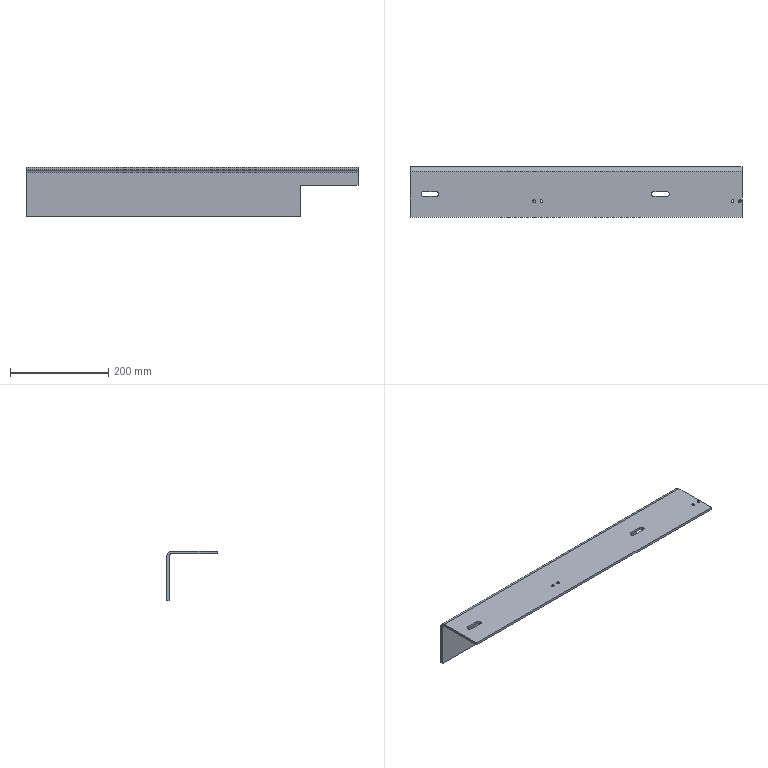Part | NX | 1 solid | 38 faces | box 677.4 x 103.1 x 101 mm | volume 622204 mm3 | cylinder 16 | plane 14 | cone 8 | commonest cylinder face diameters 5 x8 10 x7 20 x1
STEP:
#1=CARTESIAN_POINT('',(626.7,130.8,34.5));
#2=VERTEX_POINT('',#1);
#3=CARTESIAN_POINT('',(626.7,223.9,34.5));
#4=VERTEX_POINT('',#3);
#5=CARTESIAN_POINT('',(626.7,141.246,34.5));
#6=DIRECTION('',(0.,1.,0.));
#7=VECTOR('',#6,1000.);
#8=LINE('',#5,#7);
#9=EDGE_CURVE('',#2,#4,#8,.T.);
#10=ORIENTED_EDGE('',*,*,#9,.F.);
#11=CARTESIAN_POINT('',(626.7,130.8,29.5));
#12=VERTEX_POINT('',#11);
#13=CARTESIAN_POINT('',(626.7,130.8,29.5));
#14=DIRECTION('',(0.,0.,1.));
#15=VECTOR('',#14,1000.);
#16=LINE('',#13,#15);
#17=EDGE_CURVE('',#12,#2,#16,.T.);
#18=ORIENTED_EDGE('',*,*,#17,.F.);
#19=CARTESIAN_POINT('',(626.7,223.9,29.5));
#20=VERTEX_POINT('',#19);
#21=CARTESIAN_POINT('',(626.7,141.246,29.5));
#22=DIRECTION('',(0.,1.,0.));
#23=VECTOR('',#22,1000.);
#24=LINE('',#21,#23);
#25=EDGE_CURVE('',#12,#20,#24,.T.);
#26=ORIENTED_EDGE('',*,*,#25,.T.);
#27=CARTESIAN_POINT('',(626.7,228.9,24.5));
#28=VERTEX_POINT('',#27);
#29=CARTESIAN_POINT('',(626.7,223.9,24.5));
#30=DIRECTION('',(1.,0.,0.));
#31=DIRECTION('',(0.,-1.,0.));
#32=AXIS2_PLACEMENT_3D('',#29,#30,#31);
#33=CIRCLE('',#32,5.);
#34=EDGE_CURVE('',#28,#20,#33,.T.);
#35=ORIENTED_EDGE('',*,*,#34,.F.);
#36=CARTESIAN_POINT('',(626.7,228.9,-2.5));
#37=VERTEX_POINT('',#36);
#38=CARTESIAN_POINT('',(626.7,228.9,29.5));
#39=DIRECTION('',(0.,0.,-1.));
#40=VECTOR('',#39,1000.);
#41=LINE('',#38,#40);
#42=EDGE_CURVE('',#28,#37,#41,.T.);
#43=ORIENTED_EDGE('',*,*,#42,.T.);
#44=CARTESIAN_POINT('',(626.7,233.9,-2.5));
#45=VERTEX_POINT('',#44);
#46=CARTESIAN_POINT('',(626.7,141.246,-2.5));
#47=DIRECTION('',(0.,1.,0.));
#48=VECTOR('',#47,1000.);
#49=LINE('',#46,#48);
#50=EDGE_CURVE('',#37,#45,#49,.T.);
#51=ORIENTED_EDGE('',*,*,#50,.T.);
#52=CARTESIAN_POINT('',(626.7,233.9,24.5));
#53=VERTEX_POINT('',#52);
#54=CARTESIAN_POINT('',(626.7,233.9,29.5));
#55=DIRECTION('',(0.,0.,-1.));
#56=VECTOR('',#55,1000.);
#57=LINE('',#54,#56);
#58=EDGE_CURVE('',#53,#45,#57,.T.);
#59=ORIENTED_EDGE('',*,*,#58,.F.);
#60=CARTESIAN_POINT('',(626.7,223.9,24.5));
#61=DIRECTION('',(1.,0.,0.));
#62=DIRECTION('',(0.,-1.,0.));
#63=AXIS2_PLACEMENT_3D('',#60,#61,#62);
#64=CIRCLE('',#63,10.);
#65=EDGE_CURVE('',#53,#4,#64,.T.);
#66=ORIENTED_EDGE('',*,*,#65,.T.);
#67=EDGE_LOOP('',(#10,#18,#26,#35,#43,#51,#59,#66));
#68=FACE_BOUND('',#67,.T.);
#69=CARTESIAN_POINT('',(626.7,165.9,29.5));
#70=DIRECTION('',(1.,0.,0.));
#71=DIRECTION('',(0.,1.,0.));
#72=AXIS2_PLACEMENT_3D('',#69,#70,#71);
#73=PLANE('',#72);
#74=ADVANCED_FACE('',(#68),#73,.T.);
#75=CARTESIAN_POINT('',(-50.7,130.8,29.5));
#76=VERTEX_POINT('',#75);
#77=CARTESIAN_POINT('',(357.184,130.8,29.5));
#78=DIRECTION('',(1.,0.,0.));
#79=VECTOR('',#78,1000.);
#80=LINE('',#77,#79);
#81=EDGE_CURVE('',#76,#12,#80,.T.);
#82=ORIENTED_EDGE('',*,*,#81,.T.);
#83=ORIENTED_EDGE('',*,*,#17,.T.);
#84=CARTESIAN_POINT('',(-50.7,130.8,34.5));
#85=VERTEX_POINT('',#84);
#86=CARTESIAN_POINT('',(357.184,130.8,34.5));
#87=DIRECTION('',(1.,0.,0.));
#88=VECTOR('',#87,1000.);
#89=LINE('',#86,#88);
#90=EDGE_CURVE('',#85,#2,#89,.T.);
#91=ORIENTED_EDGE('',*,*,#90,.F.);
#92=CARTESIAN_POINT('',(-50.7,130.8,29.5));
#93=DIRECTION('',(0.,0.,-1.));
#94=VECTOR('',#93,1000.);
#95=LINE('',#92,#94);
#96=EDGE_CURVE('',#85,#76,#95,.T.);
#97=ORIENTED_EDGE('',*,*,#96,.T.);
#98=EDGE_LOOP('',(#82,#83,#91,#97));
#99=FACE_BOUND('',#98,.T.);
#100=CARTESIAN_POINT('',(364.7,130.8,29.5));
#101=DIRECTION('',(0.,-1.,0.));
#102=DIRECTION('',(0.,0.,-1.));
#103=AXIS2_PLACEMENT_3D('',#100,#101,#102);
#104=PLANE('',#103);
#105=ADVANCED_FACE('',(#99),#104,.T.);
#106=ORIENTED_EDGE('',*,*,#9,.T.);
#107=CARTESIAN_POINT('',(-50.7,223.9,34.5));
#108=VERTEX_POINT('',#107);
#109=CARTESIAN_POINT('',(357.184,223.9,34.5));
#110=DIRECTION('',(1.,0.,0.));
#111=VECTOR('',#110,1000.);
#112=LINE('',#109,#111);
#113=EDGE_CURVE('',#108,#4,#112,.T.);
#114=ORIENTED_EDGE('',*,*,#113,.F.);
#115=CARTESIAN_POINT('',(-50.7,141.246,34.5));
#116=DIRECTION('',(0.,-1.,0.));
#117=VECTOR('',#116,1000.);
#118=LINE('',#115,#117);
#119=EDGE_CURVE('',#108,#85,#118,.T.);
#120=ORIENTED_EDGE('',*,*,#119,.T.);
#121=ORIENTED_EDGE('',*,*,#90,.T.);
#122=EDGE_LOOP('',(#106,#114,#120,#121));
#123=FACE_BOUND('',#122,.T.);
#124=CARTESIAN_POINT('',(619.8,163.7,34.5));
#125=VERTEX_POINT('',#124);
#126=CARTESIAN_POINT('',(625.2,163.7,34.5));
#127=VERTEX_POINT('',#126);
#128=CARTESIAN_POINT('',(622.5,163.7,34.5));
#129=DIRECTION('',(0.,0.,1.));
#130=DIRECTION('',(1.,0.,0.));
#131=AXIS2_PLACEMENT_3D('',#128,#129,#130);
#132=CIRCLE('',#131,2.7);
#133=EDGE_CURVE('',#125,#127,#132,.T.);
#134=ORIENTED_EDGE('',*,*,#133,.F.);
#135=CARTESIAN_POINT('',(622.5,163.7,34.5));
#136=DIRECTION('',(0.,0.,1.));
#137=DIRECTION('',(1.,0.,0.));
#138=AXIS2_PLACEMENT_3D('',#135,#136,#137);
#139=CIRCLE('',#138,2.7);
#140=EDGE_CURVE('',#127,#125,#139,.T.);
#141=ORIENTED_EDGE('',*,*,#140,.F.);
#142=EDGE_LOOP('',(#134,#141));
#143=FACE_BOUND('',#142,.T.);
#144=CARTESIAN_POINT('',(214.8,163.7,34.5));
#145=VERTEX_POINT('',#144);
#146=CARTESIAN_POINT('',(220.2,163.7,34.5));
#147=VERTEX_POINT('',#146);
#148=CARTESIAN_POINT('',(217.5,163.7,34.5));
#149=DIRECTION('',(0.,0.,1.));
#150=DIRECTION('',(1.,0.,0.));
#151=AXIS2_PLACEMENT_3D('',#148,#149,#150);
#152=CIRCLE('',#151,2.7);
#153=EDGE_CURVE('',#145,#147,#152,.T.);
#154=ORIENTED_EDGE('',*,*,#153,.F.);
#155=CARTESIAN_POINT('',(217.5,163.7,34.5));
#156=DIRECTION('',(0.,0.,1.));
#157=DIRECTION('',(1.,0.,0.));
#158=AXIS2_PLACEMENT_3D('',#155,#156,#157);
#159=CIRCLE('',#158,2.7);
#160=EDGE_CURVE('',#147,#145,#159,.T.);
#161=ORIENTED_EDGE('',*,*,#160,.F.);
#162=EDGE_LOOP('',(#154,#161));
#163=FACE_BOUND('',#162,.T.);
#164=CARTESIAN_POINT('',(604.8,163.7,34.5));
#165=VERTEX_POINT('',#164);
#166=CARTESIAN_POINT('',(610.2,163.7,34.5));
#167=VERTEX_POINT('',#166);
#168=CARTESIAN_POINT('',(607.5,163.7,34.5));
#169=DIRECTION('',(0.,0.,1.));
#170=DIRECTION('',(1.,0.,0.));
#171=AXIS2_PLACEMENT_3D('',#168,#169,#170);
#172=CIRCLE('',#171,2.7);
#173=EDGE_CURVE('',#165,#167,#172,.T.);
#174=ORIENTED_EDGE('',*,*,#173,.F.);
#175=CARTESIAN_POINT('',(607.5,163.7,34.5));
#176=DIRECTION('',(0.,0.,1.));
#177=DIRECTION('',(1.,0.,0.));
#178=AXIS2_PLACEMENT_3D('',#175,#176,#177);
#179=CIRCLE('',#178,2.7);
#180=EDGE_CURVE('',#167,#165,#179,.T.);
#181=ORIENTED_EDGE('',*,*,#180,.F.);
#182=EDGE_LOOP('',(#174,#181));
#183=FACE_BOUND('',#182,.T.);
#184=CARTESIAN_POINT('',(199.8,163.7,34.5));
#185=VERTEX_POINT('',#184);
#186=CARTESIAN_POINT('',(205.2,163.7,34.5));
#187=VERTEX_POINT('',#186);
#188=CARTESIAN_POINT('',(202.5,163.7,34.5));
#189=DIRECTION('',(0.,0.,1.));
#190=DIRECTION('',(1.,0.,0.));
#191=AXIS2_PLACEMENT_3D('',#188,#189,#190);
#192=CIRCLE('',#191,2.7);
#193=EDGE_CURVE('',#185,#187,#192,.T.);
#194=ORIENTED_EDGE('',*,*,#193,.F.);
#195=CARTESIAN_POINT('',(202.5,163.7,34.5));
#196=DIRECTION('',(0.,0.,1.));
#197=DIRECTION('',(1.,0.,0.));
#198=AXIS2_PLACEMENT_3D('',#195,#196,#197);
#199=CIRCLE('',#198,2.7);
#200=EDGE_CURVE('',#187,#185,#199,.T.);
#201=ORIENTED_EDGE('',*,*,#200,.F.);
#202=EDGE_LOOP('',(#194,#201));
#203=FACE_BOUND('',#202,.T.);
#204=CARTESIAN_POINT('',(446.875,183.2,34.5));
#205=VERTEX_POINT('',#204);
#206=CARTESIAN_POINT('',(446.875,173.2,34.5));
#207=VERTEX_POINT('',#206);
#208=CARTESIAN_POINT('',(446.875,178.2,34.5));
#209=DIRECTION('',(0.,0.,1.));
#210=DIRECTION('',(1.,0.,0.));
#211=AXIS2_PLACEMENT_3D('',#208,#209,#210);
#212=CIRCLE('',#211,5.);
#213=EDGE_CURVE('',#205,#207,#212,.T.);
#214=ORIENTED_EDGE('',*,*,#213,.F.);
#215=CARTESIAN_POINT('',(473.125,183.2,34.5));
#216=VERTEX_POINT('',#215);
#217=CARTESIAN_POINT('',(357.184,183.2,34.5));
#218=DIRECTION('',(-1.,0.,0.));
#219=VECTOR('',#218,1000.);
#220=LINE('',#217,#219);
#221=EDGE_CURVE('',#216,#205,#220,.T.);
#222=ORIENTED_EDGE('',*,*,#221,.F.);
#223=CARTESIAN_POINT('',(478.125,178.2,34.5));
#224=VERTEX_POINT('',#223);
#225=CARTESIAN_POINT('',(473.125,178.2,34.5));
#226=DIRECTION('',(0.,0.,1.));
#227=DIRECTION('',(1.,0.,0.));
#228=AXIS2_PLACEMENT_3D('',#225,#226,#227);
#229=CIRCLE('',#228,5.);
#230=EDGE_CURVE('',#224,#216,#229,.T.);
#231=ORIENTED_EDGE('',*,*,#230,.F.);
#232=CARTESIAN_POINT('',(473.125,173.2,34.5));
#233=VERTEX_POINT('',#232);
#234=CARTESIAN_POINT('',(473.125,178.2,34.5));
#235=DIRECTION('',(0.,0.,1.));
#236=DIRECTION('',(1.,0.,0.));
#237=AXIS2_PLACEMENT_3D('',#234,#235,#236);
#238=CIRCLE('',#237,5.);
#239=EDGE_CURVE('',#233,#224,#238,.T.);
#240=ORIENTED_EDGE('',*,*,#239,.F.);
#241=CARTESIAN_POINT('',(357.184,173.2,34.5));
#242=DIRECTION('',(1.,0.,0.));
#243=VECTOR('',#242,1000.);
#244=LINE('',#241,#243);
#245=EDGE_CURVE('',#207,#233,#244,.T.);
#246=ORIENTED_EDGE('',*,*,#245,.F.);
#247=EDGE_LOOP('',(#214,#222,#231,#240,#246));
#248=FACE_BOUND('',#247,.T.);
#249=CARTESIAN_POINT('',(-23.125,183.2,34.5));
#250=VERTEX_POINT('',#249);
#251=CARTESIAN_POINT('',(-23.125,173.2,34.5));
#252=VERTEX_POINT('',#251);
#253=CARTESIAN_POINT('',(-23.125,178.2,34.5));
#254=DIRECTION('',(0.,0.,1.));
#255=DIRECTION('',(1.,0.,0.));
#256=AXIS2_PLACEMENT_3D('',#253,#254,#255);
#257=CIRCLE('',#256,5.);
#258=EDGE_CURVE('',#250,#252,#257,.T.);
#259=ORIENTED_EDGE('',*,*,#258,.F.);
#260=CARTESIAN_POINT('',(3.125,183.2,34.5));
#261=VERTEX_POINT('',#260);
#262=CARTESIAN_POINT('',(357.184,183.2,34.5));
#263=DIRECTION('',(-1.,0.,0.));
#264=VECTOR('',#263,1000.);
#265=LINE('',#262,#264);
#266=EDGE_CURVE('',#261,#250,#265,.T.);
#267=ORIENTED_EDGE('',*,*,#266,.F.);
#268=CARTESIAN_POINT('',(8.125,178.2,34.5));
#269=VERTEX_POINT('',#268);
#270=CARTESIAN_POINT('',(3.125,178.2,34.5));
#271=DIRECTION('',(0.,0.,1.));
#272=DIRECTION('',(1.,0.,0.));
#273=AXIS2_PLACEMENT_3D('',#270,#271,#272);
#274=CIRCLE('',#273,5.);
#275=EDGE_CURVE('',#269,#261,#274,.T.);
#276=ORIENTED_EDGE('',*,*,#275,.F.);
#277=CARTESIAN_POINT('',(3.125,173.2,34.5));
#278=VERTEX_POINT('',#277);
#279=CARTESIAN_POINT('',(3.125,178.2,34.5));
#280=DIRECTION('',(0.,0.,1.));
#281=DIRECTION('',(1.,0.,0.));
#282=AXIS2_PLACEMENT_3D('',#279,#280,#281);
#283=CIRCLE('',#282,5.);
#284=EDGE_CURVE('',#278,#269,#283,.T.);
#285=ORIENTED_EDGE('',*,*,#284,.F.);
#286=CARTESIAN_POINT('',(357.184,173.2,34.5));
#287=DIRECTION('',(1.,0.,0.));
#288=VECTOR('',#287,1000.);
#289=LINE('',#286,#288);
#290=EDGE_CURVE('',#252,#278,#289,.T.);
#291=ORIENTED_EDGE('',*,*,#290,.F.);
#292=EDGE_LOOP('',(#259,#267,#276,#285,#291));
#293=FACE_BOUND('',#292,.T.);
#294=CARTESIAN_POINT('',(-52.7,233.9,34.5));
#295=DIRECTION('',(0.,0.,1.));
#296=DIRECTION('',(1.,0.,0.));
#297=AXIS2_PLACEMENT_3D('',#294,#295,#296);
#298=PLANE('',#297);
#299=ADVANCED_FACE('',(#123,#143,#163,#183,#203,#248,#293),#298,.T.);
#300=CARTESIAN_POINT('',(-50.7,233.9,-66.5));
#301=VERTEX_POINT('',#300);
#302=CARTESIAN_POINT('',(-50.7,233.9,24.5));
#303=VERTEX_POINT('',#302);
#304=CARTESIAN_POINT('',(-50.7,233.9,29.5));
#305=DIRECTION('',(0.,0.,1.));
#306=VECTOR('',#305,1000.);
#307=LINE('',#304,#306);
#308=EDGE_CURVE('',#301,#303,#307,.T.);
#309=ORIENTED_EDGE('',*,*,#308,.F.);
#310=CARTESIAN_POINT('',(-50.7,228.9,-66.5));
#311=VERTEX_POINT('',#310);
#312=CARTESIAN_POINT('',(-50.7,141.246,-66.5));
#313=DIRECTION('',(0.,1.,0.));
#314=VECTOR('',#313,1000.);
#315=LINE('',#312,#314);
#316=EDGE_CURVE('',#311,#301,#315,.T.);
#317=ORIENTED_EDGE('',*,*,#316,.F.);
#318=CARTESIAN_POINT('',(-50.7,228.9,24.5));
#319=VERTEX_POINT('',#318);
#320=CARTESIAN_POINT('',(-50.7,228.9,29.5));
#321=DIRECTION('',(0.,0.,1.));
#322=VECTOR('',#321,1000.);
#323=LINE('',#320,#322);
#324=EDGE_CURVE('',#311,#319,#323,.T.);
#325=ORIENTED_EDGE('',*,*,#324,.T.);
#326=CARTESIAN_POINT('',(-50.7,223.9,29.5));
#327=VERTEX_POINT('',#326);
#328=CARTESIAN_POINT('',(-50.7,223.9,24.5));
#329=DIRECTION('',(1.,0.,0.));
#330=DIRECTION('',(0.,-1.,0.));
#331=AXIS2_PLACEMENT_3D('',#328,#329,#330);
#332=CIRCLE('',#331,5.);
#333=EDGE_CURVE('',#319,#327,#332,.T.);
#334=ORIENTED_EDGE('',*,*,#333,.T.);
#335=CARTESIAN_POINT('',(-50.7,141.246,29.5));
#336=DIRECTION('',(0.,-1.,0.));
#337=VECTOR('',#336,1000.);
#338=LINE('',#335,#337);
#339=EDGE_CURVE('',#327,#76,#338,.T.);
#340=ORIENTED_EDGE('',*,*,#339,.T.);
#341=ORIENTED_EDGE('',*,*,#96,.F.);
#342=ORIENTED_EDGE('',*,*,#119,.F.);
#343=CARTESIAN_POINT('',(-50.7,223.9,24.5));
#344=DIRECTION('',(1.,0.,0.));
#345=DIRECTION('',(0.,-1.,0.));
#346=AXIS2_PLACEMENT_3D('',#343,#344,#345);
#347=CIRCLE('',#346,10.);
#348=EDGE_CURVE('',#303,#108,#347,.T.);
#349=ORIENTED_EDGE('',*,*,#348,.F.);
#350=EDGE_LOOP('',(#309,#317,#325,#334,#340,#341,#342,#349));
#351=FACE_BOUND('',#350,.T.);
#352=CARTESIAN_POINT('',(-50.7,233.9,-60.5));
#353=DIRECTION('',(-1.,0.,0.));
#354=DIRECTION('',(0.,0.,1.));
#355=AXIS2_PLACEMENT_3D('',#352,#353,#354);
#356=PLANE('',#355);
#357=ADVANCED_FACE('',(#351),#356,.T.);
#358=CARTESIAN_POINT('',(509.7,233.9,-66.5));
#359=VERTEX_POINT('',#358);
#360=CARTESIAN_POINT('',(357.184,233.9,-66.5));
#361=DIRECTION('',(-1.,0.,0.));
#362=VECTOR('',#361,1000.);
#363=LINE('',#360,#362);
#364=EDGE_CURVE('',#359,#301,#363,.T.);
#365=ORIENTED_EDGE('',*,*,#364,.F.);
#366=CARTESIAN_POINT('',(509.7,228.9,-66.5));
#367=VERTEX_POINT('',#366);
#368=CARTESIAN_POINT('',(509.7,141.246,-66.5));
#369=DIRECTION('',(0.,1.,0.));
#370=VECTOR('',#369,1000.);
#371=LINE('',#368,#370);
#372=EDGE_CURVE('',#367,#359,#371,.T.);
#373=ORIENTED_EDGE('',*,*,#372,.F.);
#374=CARTESIAN_POINT('',(357.184,228.9,-66.5));
#375=DIRECTION('',(-1.,0.,0.));
#376=VECTOR('',#375,1000.);
#377=LINE('',#374,#376);
#378=EDGE_CURVE('',#367,#311,#377,.T.);
#379=ORIENTED_EDGE('',*,*,#378,.T.);
#380=ORIENTED_EDGE('',*,*,#316,.T.);
#381=EDGE_LOOP('',(#365,#373,#379,#380));
#382=FACE_BOUND('',#381,.T.);
#383=CARTESIAN_POINT('',(671.7,233.9,-66.5));
#384=DIRECTION('',(0.,0.,-1.));
#385=DIRECTION('',(0.,-1.,0.));
#386=AXIS2_PLACEMENT_3D('',#383,#384,#385);
#387=PLANE('',#386);
#388=ADVANCED_FACE('',(#382),#387,.T.);
#389=CARTESIAN_POINT('',(357.184,233.9,24.5));
#390=DIRECTION('',(1.,0.,0.));
#391=VECTOR('',#390,1000.);
#392=LINE('',#389,#391);
#393=EDGE_CURVE('',#303,#53,#392,.T.);
#394=ORIENTED_EDGE('',*,*,#393,.T.);
#395=ORIENTED_EDGE('',*,*,#58,.T.);
#396=CARTESIAN_POINT('',(509.7,233.9,-2.5));
#397=VERTEX_POINT('',#396);
#398=CARTESIAN_POINT('',(357.184,233.9,-2.5));
#399=DIRECTION('',(1.,0.,0.));
#400=VECTOR('',#399,1000.);
#401=LINE('',#398,#400);
#402=EDGE_CURVE('',#397,#45,#401,.T.);
#403=ORIENTED_EDGE('',*,*,#402,.F.);
#404=CARTESIAN_POINT('',(509.7,233.9,29.5));
#405=DIRECTION('',(0.,0.,1.));
#406=VECTOR('',#405,1000.);
#407=LINE('',#404,#406);
#408=EDGE_CURVE('',#359,#397,#407,.T.);
#409=ORIENTED_EDGE('',*,*,#408,.F.);
#410=ORIENTED_EDGE('',*,*,#364,.T.);
#411=ORIENTED_EDGE('',*,*,#308,.T.);
#412=EDGE_LOOP('',(#394,#395,#403,#409,#410,#411));
#413=FACE_BOUND('',#412,.T.);
#414=CARTESIAN_POINT('',(-52.7,233.9,24.907));
#415=DIRECTION('',(0.,1.,0.));
#416=DIRECTION('',(1.,0.,0.));
#417=AXIS2_PLACEMENT_3D('',#414,#415,#416);
#418=PLANE('',#417);
#419=ADVANCED_FACE('',(#413),#418,.T.);
#420=ORIENTED_EDGE('',*,*,#113,.T.);
#421=ORIENTED_EDGE('',*,*,#65,.F.);
#422=ORIENTED_EDGE('',*,*,#393,.F.);
#423=ORIENTED_EDGE('',*,*,#348,.T.);
#424=EDGE_LOOP('',(#420,#421,#422,#423));
#425=FACE_BOUND('',#424,.T.);
#426=CARTESIAN_POINT('',(671.7,223.9,24.5));
#427=DIRECTION('',(1.,0.,0.));
#428=DIRECTION('',(0.,-1.,0.));
#429=AXIS2_PLACEMENT_3D('',#426,#427,#428);
#430=CYLINDRICAL_SURFACE('',#429,10.);
#431=ADVANCED_FACE('',(#425),#430,.T.);
#432=CARTESIAN_POINT('',(605.,163.7,34.3));
#433=VERTEX_POINT('',#432);
#434=CARTESIAN_POINT('',(610.,163.7,34.3));
#435=VERTEX_POINT('',#434);
#436=CARTESIAN_POINT('',(607.5,163.7,34.3));
#437=DIRECTION('',(0.,0.,1.));
#438=DIRECTION('',(1.,0.,0.));
#439=AXIS2_PLACEMENT_3D('',#436,#437,#438);
#440=CIRCLE('',#439,2.5);
#441=EDGE_CURVE('',#433,#435,#440,.T.);
#442=ORIENTED_EDGE('',*,*,#441,.T.);
#443=CARTESIAN_POINT('',(610.,163.7,29.5));
#444=VERTEX_POINT('',#443);
#445=CARTESIAN_POINT('',(610.,163.7,34.5));
#446=DIRECTION('',(0.,0.,1.));
#447=VECTOR('',#446,1000.);
#448=LINE('',#445,#447);
#449=EDGE_CURVE('',#444,#435,#448,.T.);
#450=ORIENTED_EDGE('',*,*,#449,.F.);
#451=CARTESIAN_POINT('',(605.,163.7,29.5));
#452=VERTEX_POINT('',#451);
#453=CARTESIAN_POINT('',(607.5,163.7,29.5));
#454=DIRECTION('',(0.,0.,1.));
#455=DIRECTION('',(1.,0.,0.));
#456=AXIS2_PLACEMENT_3D('',#453,#454,#455);
#457=CIRCLE('',#456,2.5);
#458=EDGE_CURVE('',#452,#444,#457,.T.);
#459=ORIENTED_EDGE('',*,*,#458,.F.);
#460=CARTESIAN_POINT('',(605.,163.7,34.5));
#461=DIRECTION('',(0.,0.,1.));
#462=VECTOR('',#461,1000.);
#463=LINE('',#460,#462);
#464=EDGE_CURVE('',#452,#433,#463,.T.);
#465=ORIENTED_EDGE('',*,*,#464,.T.);
#466=EDGE_LOOP('',(#442,#450,#459,#465));
#467=FACE_BOUND('',#466,.T.);
#468=CARTESIAN_POINT('',(607.5,163.7,34.5));
#469=DIRECTION('',(0.,0.,1.));
#470=DIRECTION('',(1.,0.,0.));
#471=AXIS2_PLACEMENT_3D('',#468,#469,#470);
#472=CYLINDRICAL_SURFACE('',#471,2.5);
#473=ADVANCED_FACE('',(#467),#472,.F.);
#474=ORIENTED_EDGE('',*,*,#441,.F.);
#475=CARTESIAN_POINT('',(605.,163.7,34.3));
#476=DIRECTION('',(-0.7071,0.,0.7071));
#477=VECTOR('',#476,1000.);
#478=LINE('',#475,#477);
#479=EDGE_CURVE('',#433,#165,#478,.T.);
#480=ORIENTED_EDGE('',*,*,#479,.T.);
#481=ORIENTED_EDGE('',*,*,#173,.T.);
#482=CARTESIAN_POINT('',(610.,163.7,34.3));
#483=DIRECTION('',(0.7071,0.,0.7071));
#484=VECTOR('',#483,1000.);
#485=LINE('',#482,#484);
#486=EDGE_CURVE('',#435,#167,#485,.T.);
#487=ORIENTED_EDGE('',*,*,#486,.F.);
#488=EDGE_LOOP('',(#474,#480,#481,#487));
#489=FACE_BOUND('',#488,.T.);
#490=CARTESIAN_POINT('',(607.5,163.7,34.3));
#491=DIRECTION('',(0.,0.,1.));
#492=DIRECTION('',(1.,0.,0.));
#493=AXIS2_PLACEMENT_3D('',#490,#491,#492);
#494=CONICAL_SURFACE('',#493,2.5,0.7854);
#495=ADVANCED_FACE('',(#489),#494,.F.);
#496=CARTESIAN_POINT('',(200.,163.7,34.3));
#497=VERTEX_POINT('',#496);
#498=CARTESIAN_POINT('',(205.,163.7,34.3));
#499=VERTEX_POINT('',#498);
#500=CARTESIAN_POINT('',(202.5,163.7,34.3));
#501=DIRECTION('',(0.,0.,1.));
#502=DIRECTION('',(1.,0.,0.));
#503=AXIS2_PLACEMENT_3D('',#500,#501,#502);
#504=CIRCLE('',#503,2.5);
#505=EDGE_CURVE('',#497,#499,#504,.T.);
#506=ORIENTED_EDGE('',*,*,#505,.T.);
#507=CARTESIAN_POINT('',(205.,163.7,29.5));
#508=VERTEX_POINT('',#507);
#509=CARTESIAN_POINT('',(205.,163.7,34.5));
#510=DIRECTION('',(0.,0.,1.));
#511=VECTOR('',#510,1000.);
#512=LINE('',#509,#511);
#513=EDGE_CURVE('',#508,#499,#512,.T.);
#514=ORIENTED_EDGE('',*,*,#513,.F.);
#515=CARTESIAN_POINT('',(200.,163.7,29.5));
#516=VERTEX_POINT('',#515);
#517=CARTESIAN_POINT('',(202.5,163.7,29.5));
#518=DIRECTION('',(0.,0.,1.));
#519=DIRECTION('',(1.,0.,0.));
#520=AXIS2_PLACEMENT_3D('',#517,#518,#519);
#521=CIRCLE('',#520,2.5);
#522=EDGE_CURVE('',#516,#508,#521,.T.);
#523=ORIENTED_EDGE('',*,*,#522,.F.);
#524=CARTESIAN_POINT('',(200.,163.7,34.5));
#525=DIRECTION('',(0.,0.,1.));
#526=VECTOR('',#525,1000.);
#527=LINE('',#524,#526);
#528=EDGE_CURVE('',#516,#497,#527,.T.);
#529=ORIENTED_EDGE('',*,*,#528,.T.);
#530=EDGE_LOOP('',(#506,#514,#523,#529));
#531=FACE_BOUND('',#530,.T.);
#532=CARTESIAN_POINT('',(202.5,163.7,34.5));
#533=DIRECTION('',(0.,0.,1.));
#534=DIRECTION('',(1.,0.,0.));
#535=AXIS2_PLACEMENT_3D('',#532,#533,#534);
#536=CYLINDRICAL_SURFACE('',#535,2.5);
#537=ADVANCED_FACE('',(#531),#536,.F.);
#538=ORIENTED_EDGE('',*,*,#505,.F.);
#539=CARTESIAN_POINT('',(200.,163.7,34.3));
#540=DIRECTION('',(-0.7071,0.,0.7071));
#541=VECTOR('',#540,1000.);
#542=LINE('',#539,#541);
#543=EDGE_CURVE('',#497,#185,#542,.T.);
#544=ORIENTED_EDGE('',*,*,#543,.T.);
#545=ORIENTED_EDGE('',*,*,#193,.T.);
#546=CARTESIAN_POINT('',(205.,163.7,34.3));
#547=DIRECTION('',(0.7071,0.,0.7071));
#548=VECTOR('',#547,1000.);
#549=LINE('',#546,#548);
#550=EDGE_CURVE('',#499,#187,#549,.T.);
#551=ORIENTED_EDGE('',*,*,#550,.F.);
#552=EDGE_LOOP('',(#538,#544,#545,#551));
#553=FACE_BOUND('',#552,.T.);
#554=CARTESIAN_POINT('',(202.5,163.7,34.3));
#555=DIRECTION('',(0.,0.,1.));
#556=DIRECTION('',(1.,0.,0.));
#557=AXIS2_PLACEMENT_3D('',#554,#555,#556);
#558=CONICAL_SURFACE('',#557,2.5,0.7854);
#559=ADVANCED_FACE('',(#553),#558,.F.);
#560=CARTESIAN_POINT('',(215.,163.7,34.3));
#561=VERTEX_POINT('',#560);
#562=CARTESIAN_POINT('',(220.,163.7,34.3));
#563=VERTEX_POINT('',#562);
#564=CARTESIAN_POINT('',(217.5,163.7,34.3));
#565=DIRECTION('',(0.,0.,1.));
#566=DIRECTION('',(1.,0.,0.));
#567=AXIS2_PLACEMENT_3D('',#564,#565,#566);
#568=CIRCLE('',#567,2.5);
#569=EDGE_CURVE('',#561,#563,#568,.T.);
#570=ORIENTED_EDGE('',*,*,#569,.T.);
#571=CARTESIAN_POINT('',(220.,163.7,29.5));
#572=VERTEX_POINT('',#571);
#573=CARTESIAN_POINT('',(220.,163.7,34.5));
#574=DIRECTION('',(0.,0.,1.));
#575=VECTOR('',#574,1000.);
#576=LINE('',#573,#575);
#577=EDGE_CURVE('',#572,#563,#576,.T.);
#578=ORIENTED_EDGE('',*,*,#577,.F.);
#579=CARTESIAN_POINT('',(215.,163.7,29.5));
#580=VERTEX_POINT('',#579);
#581=CARTESIAN_POINT('',(217.5,163.7,29.5));
#582=DIRECTION('',(0.,0.,1.));
#583=DIRECTION('',(1.,0.,0.));
#584=AXIS2_PLACEMENT_3D('',#581,#582,#583);
#585=CIRCLE('',#584,2.5);
#586=EDGE_CURVE('',#580,#572,#585,.T.);
#587=ORIENTED_EDGE('',*,*,#586,.F.);
#588=CARTESIAN_POINT('',(215.,163.7,34.5));
#589=DIRECTION('',(0.,0.,1.));
#590=VECTOR('',#589,1000.);
#591=LINE('',#588,#590);
#592=EDGE_CURVE('',#580,#561,#591,.T.);
#593=ORIENTED_EDGE('',*,*,#592,.T.);
#594=EDGE_LOOP('',(#570,#578,#587,#593));
#595=FACE_BOUND('',#594,.T.);
#596=CARTESIAN_POINT('',(217.5,163.7,34.5));
#597=DIRECTION('',(0.,0.,1.));
#598=DIRECTION('',(1.,0.,0.));
#599=AXIS2_PLACEMENT_3D('',#596,#597,#598);
#600=CYLINDRICAL_SURFACE('',#599,2.5);
#601=ADVANCED_FACE('',(#595),#600,.F.);
#602=ORIENTED_EDGE('',*,*,#569,.F.);
#603=CARTESIAN_POINT('',(215.,163.7,34.3));
#604=DIRECTION('',(-0.7071,0.,0.7071));
#605=VECTOR('',#604,1000.);
#606=LINE('',#603,#605);
#607=EDGE_CURVE('',#561,#145,#606,.T.);
#608=ORIENTED_EDGE('',*,*,#607,.T.);
#609=ORIENTED_EDGE('',*,*,#153,.T.);
#610=CARTESIAN_POINT('',(220.,163.7,34.3));
#611=DIRECTION('',(0.7071,0.,0.7071));
#612=VECTOR('',#611,1000.);
#613=LINE('',#610,#612);
#614=EDGE_CURVE('',#563,#147,#613,.T.);
#615=ORIENTED_EDGE('',*,*,#614,.F.);
#616=EDGE_LOOP('',(#602,#608,#609,#615));
#617=FACE_BOUND('',#616,.T.);
#618=CARTESIAN_POINT('',(217.5,163.7,34.3));
#619=DIRECTION('',(0.,0.,1.));
#620=DIRECTION('',(1.,0.,0.));
#621=AXIS2_PLACEMENT_3D('',#618,#619,#620);
#622=CONICAL_SURFACE('',#621,2.5,0.7854);
#623=ADVANCED_FACE('',(#617),#622,.F.);
#624=CARTESIAN_POINT('',(478.125,178.2,29.5));
#625=VERTEX_POINT('',#624);
#626=CARTESIAN_POINT('',(478.125,178.2,-76.6));
#627=DIRECTION('',(0.,0.,1.));
#628=VECTOR('',#627,1000.);
#629=LINE('',#626,#628);
#630=EDGE_CURVE('',#625,#224,#629,.T.);
#631=ORIENTED_EDGE('',*,*,#630,.F.);
#632=CARTESIAN_POINT('',(473.125,173.2,29.5));
#633=VERTEX_POINT('',#632);
#634=CARTESIAN_POINT('',(473.125,178.2,29.5));
#635=DIRECTION('',(0.,0.,1.));
#636=DIRECTION('',(1.,0.,0.));
#637=AXIS2_PLACEMENT_3D('',#634,#635,#636);
#638=CIRCLE('',#637,5.);
#639=EDGE_CURVE('',#633,#625,#638,.T.);
#640=ORIENTED_EDGE('',*,*,#639,.F.);
#641=CARTESIAN_POINT('',(473.125,173.2,-76.6));
#642=DIRECTION('',(0.,0.,1.));
#643=VECTOR('',#642,1000.);
#644=LINE('',#641,#643);
#645=EDGE_CURVE('',#633,#233,#644,.T.);
#646=ORIENTED_EDGE('',*,*,#645,.T.);
#647=ORIENTED_EDGE('',*,*,#239,.T.);
#648=EDGE_LOOP('',(#631,#640,#646,#647));
#649=FACE_BOUND('',#648,.T.);
#650=CARTESIAN_POINT('',(473.125,178.2,-76.6));
#651=DIRECTION('',(0.,0.,1.));
#652=DIRECTION('',(1.,0.,0.));
#653=AXIS2_PLACEMENT_3D('',#650,#651,#652);
#654=CYLINDRICAL_SURFACE('',#653,5.);
#655=ADVANCED_FACE('',(#649),#654,.F.);
#656=ORIENTED_EDGE('',*,*,#221,.T.);
#657=CARTESIAN_POINT('',(446.875,183.2,29.5));
#658=VERTEX_POINT('',#657);
#659=CARTESIAN_POINT('',(446.875,183.2,-76.6));
#660=DIRECTION('',(0.,0.,1.));
#661=VECTOR('',#660,1000.);
#662=LINE('',#659,#661);
#663=EDGE_CURVE('',#658,#205,#662,.T.);
#664=ORIENTED_EDGE('',*,*,#663,.F.);
#665=CARTESIAN_POINT('',(473.125,183.2,29.5));
#666=VERTEX_POINT('',#665);
#667=CARTESIAN_POINT('',(357.184,183.2,29.5));
#668=DIRECTION('',(-1.,0.,0.));
#669=VECTOR('',#668,1000.);
#670=LINE('',#667,#669);
#671=EDGE_CURVE('',#666,#658,#670,.T.);
#672=ORIENTED_EDGE('',*,*,#671,.F.);
#673=CARTESIAN_POINT('',(473.125,183.2,-76.6));
#674=DIRECTION('',(0.,0.,1.));
#675=VECTOR('',#674,1000.);
#676=LINE('',#673,#675);
#677=EDGE_CURVE('',#666,#216,#676,.T.);
#678=ORIENTED_EDGE('',*,*,#677,.T.);
#679=EDGE_LOOP('',(#656,#664,#672,#678));
#680=FACE_BOUND('',#679,.T.);
#681=CARTESIAN_POINT('',(446.875,183.2,-76.6));
#682=DIRECTION('',(0.,1.,0.));
#683=DIRECTION('',(1.,0.,0.));
#684=AXIS2_PLACEMENT_3D('',#681,#682,#683);
#685=PLANE('',#684);
#686=ADVANCED_FACE('',(#680),#685,.F.);
#687=ORIENTED_EDGE('',*,*,#213,.T.);
#688=CARTESIAN_POINT('',(446.875,173.2,29.5));
#689=VERTEX_POINT('',#688);
#690=CARTESIAN_POINT('',(446.875,173.2,-76.6));
#691=DIRECTION('',(0.,0.,1.));
#692=VECTOR('',#691,1000.);
#693=LINE('',#690,#692);
#694=EDGE_CURVE('',#689,#207,#693,.T.);
#695=ORIENTED_EDGE('',*,*,#694,.F.);
#696=CARTESIAN_POINT('',(446.875,178.2,29.5));
#697=DIRECTION('',(0.,0.,1.));
#698=DIRECTION('',(1.,0.,0.));
#699=AXIS2_PLACEMENT_3D('',#696,#697,#698);
#700=CIRCLE('',#699,5.);
#701=EDGE_CURVE('',#658,#689,#700,.T.);
#702=ORIENTED_EDGE('',*,*,#701,.F.);
#703=ORIENTED_EDGE('',*,*,#663,.T.);
#704=EDGE_LOOP('',(#687,#695,#702,#703));
#705=FACE_BOUND('',#704,.T.);
#706=CARTESIAN_POINT('',(446.875,178.2,-76.6));
#707=DIRECTION('',(0.,0.,1.));
#708=DIRECTION('',(1.,0.,0.));
#709=AXIS2_PLACEMENT_3D('',#706,#707,#708);
#710=CYLINDRICAL_SURFACE('',#709,5.);
#711=ADVANCED_FACE('',(#705),#710,.F.);
#712=ORIENTED_EDGE('',*,*,#245,.T.);
#713=ORIENTED_EDGE('',*,*,#645,.F.);
#714=CARTESIAN_POINT('',(357.184,173.2,29.5));
#715=DIRECTION('',(1.,0.,0.));
#716=VECTOR('',#715,1000.);
#717=LINE('',#714,#716);
#718=EDGE_CURVE('',#689,#633,#717,.T.);
#719=ORIENTED_EDGE('',*,*,#718,.F.);
#720=ORIENTED_EDGE('',*,*,#694,.T.);
#721=EDGE_LOOP('',(#712,#713,#719,#720));
#722=FACE_BOUND('',#721,.T.);
#723=CARTESIAN_POINT('',(473.125,173.2,-76.6));
#724=DIRECTION('',(0.,-1.,0.));
#725=DIRECTION('',(0.,0.,-1.));
#726=AXIS2_PLACEMENT_3D('',#723,#724,#725);
#727=PLANE('',#726);
#728=ADVANCED_FACE('',(#722),#727,.F.);
#729=CARTESIAN_POINT('',(8.125,178.2,29.5));
#730=VERTEX_POINT('',#729);
#731=CARTESIAN_POINT('',(8.125,178.2,-76.6));
#732=DIRECTION('',(0.,0.,1.));
#733=VECTOR('',#732,1000.);
#734=LINE('',#731,#733);
#735=EDGE_CURVE('',#730,#269,#734,.T.);
#736=ORIENTED_EDGE('',*,*,#735,.F.);
#737=CARTESIAN_POINT('',(3.125,173.2,29.5));
#738=VERTEX_POINT('',#737);
#739=CARTESIAN_POINT('',(3.125,178.2,29.5));
#740=DIRECTION('',(0.,0.,1.));
#741=DIRECTION('',(1.,0.,0.));
#742=AXIS2_PLACEMENT_3D('',#739,#740,#741);
#743=CIRCLE('',#742,5.);
#744=EDGE_CURVE('',#738,#730,#743,.T.);
#745=ORIENTED_EDGE('',*,*,#744,.F.);
#746=CARTESIAN_POINT('',(3.125,173.2,-76.6));
#747=DIRECTION('',(0.,0.,1.));
#748=VECTOR('',#747,1000.);
#749=LINE('',#746,#748);
#750=EDGE_CURVE('',#738,#278,#749,.T.);
#751=ORIENTED_EDGE('',*,*,#750,.T.);
#752=ORIENTED_EDGE('',*,*,#284,.T.);
#753=EDGE_LOOP('',(#736,#745,#751,#752));
#754=FACE_BOUND('',#753,.T.);
#755=CARTESIAN_POINT('',(3.125,178.2,-76.6));
#756=DIRECTION('',(0.,0.,1.));
#757=DIRECTION('',(1.,0.,0.));
#758=AXIS2_PLACEMENT_3D('',#755,#756,#757);
#759=CYLINDRICAL_SURFACE('',#758,5.);
#760=ADVANCED_FACE('',(#754),#759,.F.);
#761=CARTESIAN_POINT('',(3.125,183.2,29.5));
#762=VERTEX_POINT('',#761);
#763=CARTESIAN_POINT('',(-23.125,183.2,29.5));
#764=VERTEX_POINT('',#763);
#765=CARTESIAN_POINT('',(357.184,183.2,29.5));
#766=DIRECTION('',(-1.,0.,0.));
#767=VECTOR('',#766,1000.);
#768=LINE('',#765,#767);
#769=EDGE_CURVE('',#762,#764,#768,.T.);
#770=ORIENTED_EDGE('',*,*,#769,.F.);
#771=CARTESIAN_POINT('',(3.125,183.2,-76.6));
#772=DIRECTION('',(0.,0.,1.));
#773=VECTOR('',#772,1000.);
#774=LINE('',#771,#773);
#775=EDGE_CURVE('',#762,#261,#774,.T.);
#776=ORIENTED_EDGE('',*,*,#775,.T.);
#777=ORIENTED_EDGE('',*,*,#266,.T.);
#778=CARTESIAN_POINT('',(-23.125,183.2,-76.6));
#779=DIRECTION('',(0.,0.,1.));
#780=VECTOR('',#779,1000.);
#781=LINE('',#778,#780);
#782=EDGE_CURVE('',#764,#250,#781,.T.);
#783=ORIENTED_EDGE('',*,*,#782,.F.);
#784=EDGE_LOOP('',(#770,#776,#777,#783));
#785=FACE_BOUND('',#784,.T.);
#786=CARTESIAN_POINT('',(-23.125,183.2,-76.6));
#787=DIRECTION('',(0.,1.,0.));
#788=DIRECTION('',(1.,0.,0.));
#789=AXIS2_PLACEMENT_3D('',#786,#787,#788);
#790=PLANE('',#789);
#791=ADVANCED_FACE('',(#785),#790,.F.);
#792=ORIENTED_EDGE('',*,*,#258,.T.);
#793=CARTESIAN_POINT('',(-23.125,173.2,29.5));
#794=VERTEX_POINT('',#793);
#795=CARTESIAN_POINT('',(-23.125,173.2,-76.6));
#796=DIRECTION('',(0.,0.,1.));
#797=VECTOR('',#796,1000.);
#798=LINE('',#795,#797);
#799=EDGE_CURVE('',#794,#252,#798,.T.);
#800=ORIENTED_EDGE('',*,*,#799,.F.);
#801=CARTESIAN_POINT('',(-23.125,178.2,29.5));
#802=DIRECTION('',(0.,0.,1.));
#803=DIRECTION('',(1.,0.,0.));
#804=AXIS2_PLACEMENT_3D('',#801,#802,#803);
#805=CIRCLE('',#804,5.);
#806=EDGE_CURVE('',#764,#794,#805,.T.);
#807=ORIENTED_EDGE('',*,*,#806,.F.);
#808=ORIENTED_EDGE('',*,*,#782,.T.);
#809=EDGE_LOOP('',(#792,#800,#807,#808));
#810=FACE_BOUND('',#809,.T.);
#811=CARTESIAN_POINT('',(-23.125,178.2,-76.6));
#812=DIRECTION('',(0.,0.,1.));
#813=DIRECTION('',(1.,0.,0.));
#814=AXIS2_PLACEMENT_3D('',#811,#812,#813);
#815=CYLINDRICAL_SURFACE('',#814,5.);
#816=ADVANCED_FACE('',(#810),#815,.F.);
#817=CARTESIAN_POINT('',(357.184,173.2,29.5));
#818=DIRECTION('',(1.,0.,0.));
#819=VECTOR('',#818,1000.);
#820=LINE('',#817,#819);
#821=EDGE_CURVE('',#794,#738,#820,.T.);
#822=ORIENTED_EDGE('',*,*,#821,.F.);
#823=ORIENTED_EDGE('',*,*,#799,.T.);
#824=ORIENTED_EDGE('',*,*,#290,.T.);
#825=ORIENTED_EDGE('',*,*,#750,.F.);
#826=EDGE_LOOP('',(#822,#823,#824,#825));
#827=FACE_BOUND('',#826,.T.);
#828=CARTESIAN_POINT('',(3.125,173.2,-76.6));
#829=DIRECTION('',(0.,-1.,0.));
#830=DIRECTION('',(0.,0.,-1.));
#831=AXIS2_PLACEMENT_3D('',#828,#829,#830);
#832=PLANE('',#831);
#833=ADVANCED_FACE('',(#827),#832,.F.);
#834=ORIENTED_EDGE('',*,*,#614,.T.);
#835=ORIENTED_EDGE('',*,*,#160,.T.);
#836=ORIENTED_EDGE('',*,*,#607,.F.);
#837=CARTESIAN_POINT('',(217.5,163.7,34.3));
#838=DIRECTION('',(0.,0.,1.));
#839=DIRECTION('',(1.,0.,0.));
#840=AXIS2_PLACEMENT_3D('',#837,#838,#839);
#841=CIRCLE('',#840,2.5);
#842=EDGE_CURVE('',#563,#561,#841,.T.);
#843=ORIENTED_EDGE('',*,*,#842,.F.);
#844=EDGE_LOOP('',(#834,#835,#836,#843));
#845=FACE_BOUND('',#844,.T.);
#846=CARTESIAN_POINT('',(217.5,163.7,34.3));
#847=DIRECTION('',(0.,0.,1.));
#848=DIRECTION('',(1.,0.,0.));
#849=AXIS2_PLACEMENT_3D('',#846,#847,#848);
#850=CONICAL_SURFACE('',#849,2.5,0.7854);
#851=ADVANCED_FACE('',(#845),#850,.F.);
#852=ORIENTED_EDGE('',*,*,#449,.T.);
#853=CARTESIAN_POINT('',(607.5,163.7,34.3));
#854=DIRECTION('',(0.,0.,1.));
#855=DIRECTION('',(1.,0.,0.));
#856=AXIS2_PLACEMENT_3D('',#853,#854,#855);
#857=CIRCLE('',#856,2.5);
#858=EDGE_CURVE('',#435,#433,#857,.T.);
#859=ORIENTED_EDGE('',*,*,#858,.T.);
#860=ORIENTED_EDGE('',*,*,#464,.F.);
#861=CARTESIAN_POINT('',(607.5,163.7,29.5));
#862=DIRECTION('',(0.,0.,1.));
#863=DIRECTION('',(1.,0.,0.));
#864=AXIS2_PLACEMENT_3D('',#861,#862,#863);
#865=CIRCLE('',#864,2.5);
#866=EDGE_CURVE('',#444,#452,#865,.T.);
#867=ORIENTED_EDGE('',*,*,#866,.F.);
#868=EDGE_LOOP('',(#852,#859,#860,#867));
#869=FACE_BOUND('',#868,.T.);
#870=CARTESIAN_POINT('',(607.5,163.7,34.5));
#871=DIRECTION('',(0.,0.,1.));
#872=DIRECTION('',(1.,0.,0.));
#873=AXIS2_PLACEMENT_3D('',#870,#871,#872);
#874=CYLINDRICAL_SURFACE('',#873,2.5);
#875=ADVANCED_FACE('',(#869),#874,.F.);
#876=ORIENTED_EDGE('',*,*,#577,.T.);
#877=ORIENTED_EDGE('',*,*,#842,.T.);
#878=ORIENTED_EDGE('',*,*,#592,.F.);
#879=CARTESIAN_POINT('',(217.5,163.7,29.5));
#880=DIRECTION('',(0.,0.,1.));
#881=DIRECTION('',(1.,0.,0.));
#882=AXIS2_PLACEMENT_3D('',#879,#880,#881);
#883=CIRCLE('',#882,2.5);
#884=EDGE_CURVE('',#572,#580,#883,.T.);
#885=ORIENTED_EDGE('',*,*,#884,.F.);
#886=EDGE_LOOP('',(#876,#877,#878,#885));
#887=FACE_BOUND('',#886,.T.);
#888=CARTESIAN_POINT('',(217.5,163.7,34.5));
#889=DIRECTION('',(0.,0.,1.));
#890=DIRECTION('',(1.,0.,0.));
#891=AXIS2_PLACEMENT_3D('',#888,#889,#890);
#892=CYLINDRICAL_SURFACE('',#891,2.5);
#893=ADVANCED_FACE('',(#887),#892,.F.);
#894=ORIENTED_EDGE('',*,*,#486,.T.);
#895=ORIENTED_EDGE('',*,*,#180,.T.);
#896=ORIENTED_EDGE('',*,*,#479,.F.);
#897=ORIENTED_EDGE('',*,*,#858,.F.);
#898=EDGE_LOOP('',(#894,#895,#896,#897));
#899=FACE_BOUND('',#898,.T.);
#900=CARTESIAN_POINT('',(607.5,163.7,34.3));
#901=DIRECTION('',(0.,0.,1.));
#902=DIRECTION('',(1.,0.,0.));
#903=AXIS2_PLACEMENT_3D('',#900,#901,#902);
#904=CONICAL_SURFACE('',#903,2.5,0.7854);
#905=ADVANCED_FACE('',(#899),#904,.F.);
#906=ORIENTED_EDGE('',*,*,#550,.T.);
#907=ORIENTED_EDGE('',*,*,#200,.T.);
#908=ORIENTED_EDGE('',*,*,#543,.F.);
#909=CARTESIAN_POINT('',(202.5,163.7,34.3));
#910=DIRECTION('',(0.,0.,1.));
#911=DIRECTION('',(1.,0.,0.));
#912=AXIS2_PLACEMENT_3D('',#909,#910,#911);
#913=CIRCLE('',#912,2.5);
#914=EDGE_CURVE('',#499,#497,#913,.T.);
#915=ORIENTED_EDGE('',*,*,#914,.F.);
#916=EDGE_LOOP('',(#906,#907,#908,#915));
#917=FACE_BOUND('',#916,.T.);
#918=CARTESIAN_POINT('',(202.5,163.7,34.3));
#919=DIRECTION('',(0.,0.,1.));
#920=DIRECTION('',(1.,0.,0.));
#921=AXIS2_PLACEMENT_3D('',#918,#919,#920);
#922=CONICAL_SURFACE('',#921,2.5,0.7854);
#923=ADVANCED_FACE('',(#917),#922,.F.);
#924=ORIENTED_EDGE('',*,*,#513,.T.);
#925=ORIENTED_EDGE('',*,*,#914,.T.);
#926=ORIENTED_EDGE('',*,*,#528,.F.);
#927=CARTESIAN_POINT('',(202.5,163.7,29.5));
#928=DIRECTION('',(0.,0.,1.));
#929=DIRECTION('',(1.,0.,0.));
#930=AXIS2_PLACEMENT_3D('',#927,#928,#929);
#931=CIRCLE('',#930,2.5);
#932=EDGE_CURVE('',#508,#516,#931,.T.);
#933=ORIENTED_EDGE('',*,*,#932,.F.);
#934=EDGE_LOOP('',(#924,#925,#926,#933));
#935=FACE_BOUND('',#934,.T.);
#936=CARTESIAN_POINT('',(202.5,163.7,34.5));
#937=DIRECTION('',(0.,0.,1.));
#938=DIRECTION('',(1.,0.,0.));
#939=AXIS2_PLACEMENT_3D('',#936,#937,#938);
#940=CYLINDRICAL_SURFACE('',#939,2.5);
#941=ADVANCED_FACE('',(#935),#940,.F.);
#942=CARTESIAN_POINT('',(509.7,228.9,-2.5));
#943=VERTEX_POINT('',#942);
#944=CARTESIAN_POINT('',(509.7,228.9,29.5));
#945=DIRECTION('',(0.,0.,1.));
#946=VECTOR('',#945,1000.);
#947=LINE('',#944,#946);
#948=EDGE_CURVE('',#367,#943,#947,.T.);
#949=ORIENTED_EDGE('',*,*,#948,.T.);
#950=CARTESIAN_POINT('',(357.184,228.9,-2.5));
#951=DIRECTION('',(1.,0.,0.));
#952=VECTOR('',#951,1000.);
#953=LINE('',#950,#952);
#954=EDGE_CURVE('',#943,#37,#953,.T.);
#955=ORIENTED_EDGE('',*,*,#954,.T.);
#956=ORIENTED_EDGE('',*,*,#42,.F.);
#957=CARTESIAN_POINT('',(357.184,228.9,24.5));
#958=DIRECTION('',(1.,0.,0.));
#959=VECTOR('',#958,1000.);
#960=LINE('',#957,#959);
#961=EDGE_CURVE('',#319,#28,#960,.T.);
#962=ORIENTED_EDGE('',*,*,#961,.F.);
#963=ORIENTED_EDGE('',*,*,#324,.F.);
#964=ORIENTED_EDGE('',*,*,#378,.F.);
#965=EDGE_LOOP('',(#949,#955,#956,#962,#963,#964));
#966=FACE_BOUND('',#965,.T.);
#967=CARTESIAN_POINT('',(357.184,228.9,117.561));
#968=DIRECTION('',(0.,1.,0.));
#969=DIRECTION('',(1.,0.,0.));
#970=AXIS2_PLACEMENT_3D('',#967,#968,#969);
#971=PLANE('',#970);
#972=ADVANCED_FACE('',(#966),#971,.F.);
#973=CARTESIAN_POINT('',(357.184,223.9,29.5));
#974=DIRECTION('',(1.,0.,0.));
#975=VECTOR('',#974,1000.);
#976=LINE('',#973,#975);
#977=EDGE_CURVE('',#327,#20,#976,.T.);
#978=ORIENTED_EDGE('',*,*,#977,.T.);
#979=ORIENTED_EDGE('',*,*,#25,.F.);
#980=ORIENTED_EDGE('',*,*,#81,.F.);
#981=ORIENTED_EDGE('',*,*,#339,.F.);
#982=EDGE_LOOP('',(#978,#979,#980,#981));
#983=FACE_BOUND('',#982,.T.);
#984=CARTESIAN_POINT('',(620.,163.7,29.5));
#985=VERTEX_POINT('',#984);
#986=CARTESIAN_POINT('',(625.,163.7,29.5));
#987=VERTEX_POINT('',#986);
#988=CARTESIAN_POINT('',(622.5,163.7,29.5));
#989=DIRECTION('',(0.,0.,1.));
#990=DIRECTION('',(1.,0.,0.));
#991=AXIS2_PLACEMENT_3D('',#988,#989,#990);
#992=CIRCLE('',#991,2.5);
#993=EDGE_CURVE('',#985,#987,#992,.T.);
#994=ORIENTED_EDGE('',*,*,#993,.T.);
#995=CARTESIAN_POINT('',(622.5,163.7,29.5));
#996=DIRECTION('',(0.,0.,1.));
#997=DIRECTION('',(1.,0.,0.));
#998=AXIS2_PLACEMENT_3D('',#995,#996,#997);
#999=CIRCLE('',#998,2.5);
#1000=EDGE_CURVE('',#987,#985,#999,.T.);
#1001=ORIENTED_EDGE('',*,*,#1000,.T.);
#1002=EDGE_LOOP('',(#994,#1001));
#1003=FACE_BOUND('',#1002,.T.);
#1004=ORIENTED_EDGE('',*,*,#522,.T.);
#1005=ORIENTED_EDGE('',*,*,#932,.T.);
#1006=EDGE_LOOP('',(#1004,#1005));
#1007=FACE_BOUND('',#1006,.T.);
#1008=ORIENTED_EDGE('',*,*,#586,.T.);
#1009=ORIENTED_EDGE('',*,*,#884,.T.);
#1010=EDGE_LOOP('',(#1008,#1009));
#1011=FACE_BOUND('',#1010,.T.);
#1012=ORIENTED_EDGE('',*,*,#458,.T.);
#1013=ORIENTED_EDGE('',*,*,#866,.T.);
#1014=EDGE_LOOP('',(#1012,#1013));
#1015=FACE_BOUND('',#1014,.T.);
#1016=ORIENTED_EDGE('',*,*,#701,.T.);
#1017=ORIENTED_EDGE('',*,*,#718,.T.);
#1018=ORIENTED_EDGE('',*,*,#639,.T.);
#1019=CARTESIAN_POINT('',(473.125,178.2,29.5));
#1020=DIRECTION('',(0.,0.,1.));
#1021=DIRECTION('',(1.,0.,0.));
#1022=AXIS2_PLACEMENT_3D('',#1019,#1020,#1021);
#1023=CIRCLE('',#1022,5.);
#1024=EDGE_CURVE('',#625,#666,#1023,.T.);
#1025=ORIENTED_EDGE('',*,*,#1024,.T.);
#1026=ORIENTED_EDGE('',*,*,#671,.T.);
#1027=EDGE_LOOP('',(#1016,#1017,#1018,#1025,#1026));
#1028=FACE_BOUND('',#1027,.T.);
#1029=ORIENTED_EDGE('',*,*,#806,.T.);
#1030=ORIENTED_EDGE('',*,*,#821,.T.);
#1031=ORIENTED_EDGE('',*,*,#744,.T.);
#1032=CARTESIAN_POINT('',(3.125,178.2,29.5));
#1033=DIRECTION('',(0.,0.,1.));
#1034=DIRECTION('',(1.,0.,0.));
#1035=AXIS2_PLACEMENT_3D('',#1032,#1033,#1034);
#1036=CIRCLE('',#1035,5.);
#1037=EDGE_CURVE('',#730,#762,#1036,.T.);
#1038=ORIENTED_EDGE('',*,*,#1037,.T.);
#1039=ORIENTED_EDGE('',*,*,#769,.T.);
#1040=EDGE_LOOP('',(#1029,#1030,#1031,#1038,#1039));
#1041=FACE_BOUND('',#1040,.T.);
#1042=CARTESIAN_POINT('',(357.184,141.246,29.5));
#1043=DIRECTION('',(0.,0.,1.));
#1044=DIRECTION('',(1.,0.,0.));
#1045=AXIS2_PLACEMENT_3D('',#1042,#1043,#1044);
#1046=PLANE('',#1045);
#1047=ADVANCED_FACE('',(#983,#1003,#1007,#1011,#1015,#1028,#1041),#1046,.F.);
#1048=ORIENTED_EDGE('',*,*,#961,.T.);
#1049=ORIENTED_EDGE('',*,*,#34,.T.);
#1050=ORIENTED_EDGE('',*,*,#977,.F.);
#1051=ORIENTED_EDGE('',*,*,#333,.F.);
#1052=EDGE_LOOP('',(#1048,#1049,#1050,#1051));
#1053=FACE_BOUND('',#1052,.T.);
#1054=CARTESIAN_POINT('',(671.7,223.9,24.5));
#1055=DIRECTION('',(1.,0.,0.));
#1056=DIRECTION('',(0.,-1.,0.));
#1057=AXIS2_PLACEMENT_3D('',#1054,#1055,#1056);
#1058=CYLINDRICAL_SURFACE('',#1057,5.);
#1059=ADVANCED_FACE('',(#1053),#1058,.F.);
#1060=ORIENTED_EDGE('',*,*,#954,.F.);
#1061=CARTESIAN_POINT('',(509.7,141.246,-2.5));
#1062=DIRECTION('',(0.,-1.,0.));
#1063=VECTOR('',#1062,1000.);
#1064=LINE('',#1061,#1063);
#1065=EDGE_CURVE('',#397,#943,#1064,.T.);
#1066=ORIENTED_EDGE('',*,*,#1065,.F.);
#1067=ORIENTED_EDGE('',*,*,#402,.T.);
#1068=ORIENTED_EDGE('',*,*,#50,.F.);
#1069=EDGE_LOOP('',(#1060,#1066,#1067,#1068));
#1070=FACE_BOUND('',#1069,.T.);
#1071=CARTESIAN_POINT('',(625.7,120.49,-2.5));
#1072=DIRECTION('',(0.,0.,1.));
#1073=DIRECTION('',(1.,0.,0.));
#1074=AXIS2_PLACEMENT_3D('',#1071,#1072,#1073);
#1075=PLANE('',#1074);
#1076=ADVANCED_FACE('',(#1070),#1075,.F.);
#1077=ORIENTED_EDGE('',*,*,#948,.F.);
#1078=ORIENTED_EDGE('',*,*,#372,.T.);
#1079=ORIENTED_EDGE('',*,*,#408,.T.);
#1080=ORIENTED_EDGE('',*,*,#1065,.T.);
#1081=EDGE_LOOP('',(#1077,#1078,#1079,#1080));
#1082=FACE_BOUND('',#1081,.T.);
#1083=CARTESIAN_POINT('',(509.7,120.49,1.5));
#1084=DIRECTION('',(-1.,0.,0.));
#1085=DIRECTION('',(0.,0.,1.));
#1086=AXIS2_PLACEMENT_3D('',#1083,#1084,#1085);
#1087=PLANE('',#1086);
#1088=ADVANCED_FACE('',(#1082),#1087,.F.);
#1089=CARTESIAN_POINT('',(620.,163.7,34.3));
#1090=VERTEX_POINT('',#1089);
#1091=CARTESIAN_POINT('',(625.,163.7,34.3));
#1092=VERTEX_POINT('',#1091);
#1093=CARTESIAN_POINT('',(622.5,163.7,34.3));
#1094=DIRECTION('',(0.,0.,1.));
#1095=DIRECTION('',(1.,0.,0.));
#1096=AXIS2_PLACEMENT_3D('',#1093,#1094,#1095);
#1097=CIRCLE('',#1096,2.5);
#1098=EDGE_CURVE('',#1090,#1092,#1097,.T.);
#1099=ORIENTED_EDGE('',*,*,#1098,.T.);
#1100=CARTESIAN_POINT('',(625.,163.7,34.5));
#1101=DIRECTION('',(0.,0.,1.));
#1102=VECTOR('',#1101,1000.);
#1103=LINE('',#1100,#1102);
#1104=EDGE_CURVE('',#987,#1092,#1103,.T.);
#1105=ORIENTED_EDGE('',*,*,#1104,.F.);
#1106=ORIENTED_EDGE('',*,*,#993,.F.);
#1107=CARTESIAN_POINT('',(620.,163.7,34.5));
#1108=DIRECTION('',(0.,0.,1.));
#1109=VECTOR('',#1108,1000.);
#1110=LINE('',#1107,#1109);
#1111=EDGE_CURVE('',#985,#1090,#1110,.T.);
#1112=ORIENTED_EDGE('',*,*,#1111,.T.);
#1113=EDGE_LOOP('',(#1099,#1105,#1106,#1112));
#1114=FACE_BOUND('',#1113,.T.);
#1115=CARTESIAN_POINT('',(622.5,163.7,34.5));
#1116=DIRECTION('',(0.,0.,1.));
#1117=DIRECTION('',(1.,0.,0.));
#1118=AXIS2_PLACEMENT_3D('',#1115,#1116,#1117);
#1119=CYLINDRICAL_SURFACE('',#1118,2.5);
#1120=ADVANCED_FACE('',(#1114),#1119,.F.);
#1121=ORIENTED_EDGE('',*,*,#1098,.F.);
#1122=CARTESIAN_POINT('',(620.,163.7,34.3));
#1123=DIRECTION('',(-0.7071,0.,0.7071));
#1124=VECTOR('',#1123,1000.);
#1125=LINE('',#1122,#1124);
#1126=EDGE_CURVE('',#1090,#125,#1125,.T.);
#1127=ORIENTED_EDGE('',*,*,#1126,.T.);
#1128=ORIENTED_EDGE('',*,*,#133,.T.);
#1129=CARTESIAN_POINT('',(625.,163.7,34.3));
#1130=DIRECTION('',(0.7071,0.,0.7071));
#1131=VECTOR('',#1130,1000.);
#1132=LINE('',#1129,#1131);
#1133=EDGE_CURVE('',#1092,#127,#1132,.T.);
#1134=ORIENTED_EDGE('',*,*,#1133,.F.);
#1135=EDGE_LOOP('',(#1121,#1127,#1128,#1134));
#1136=FACE_BOUND('',#1135,.T.);
#1137=CARTESIAN_POINT('',(622.5,163.7,34.3));
#1138=DIRECTION('',(0.,0.,1.));
#1139=DIRECTION('',(1.,0.,0.));
#1140=AXIS2_PLACEMENT_3D('',#1137,#1138,#1139);
#1141=CONICAL_SURFACE('',#1140,2.5,0.7854);
#1142=ADVANCED_FACE('',(#1136),#1141,.F.);
#1143=ORIENTED_EDGE('',*,*,#1133,.T.);
#1144=ORIENTED_EDGE('',*,*,#140,.T.);
#1145=ORIENTED_EDGE('',*,*,#1126,.F.);
#1146=CARTESIAN_POINT('',(622.5,163.7,34.3));
#1147=DIRECTION('',(0.,0.,1.));
#1148=DIRECTION('',(1.,0.,0.));
#1149=AXIS2_PLACEMENT_3D('',#1146,#1147,#1148);
#1150=CIRCLE('',#1149,2.5);
#1151=EDGE_CURVE('',#1092,#1090,#1150,.T.);
#1152=ORIENTED_EDGE('',*,*,#1151,.F.);
#1153=EDGE_LOOP('',(#1143,#1144,#1145,#1152));
#1154=FACE_BOUND('',#1153,.T.);
#1155=CARTESIAN_POINT('',(622.5,163.7,34.3));
#1156=DIRECTION('',(0.,0.,1.));
#1157=DIRECTION('',(1.,0.,0.));
#1158=AXIS2_PLACEMENT_3D('',#1155,#1156,#1157);
#1159=CONICAL_SURFACE('',#1158,2.5,0.7854);
#1160=ADVANCED_FACE('',(#1154),#1159,.F.);
#1161=ORIENTED_EDGE('',*,*,#1104,.T.);
#1162=ORIENTED_EDGE('',*,*,#1151,.T.);
#1163=ORIENTED_EDGE('',*,*,#1111,.F.);
#1164=ORIENTED_EDGE('',*,*,#1000,.F.);
#1165=EDGE_LOOP('',(#1161,#1162,#1163,#1164));
#1166=FACE_BOUND('',#1165,.T.);
#1167=CARTESIAN_POINT('',(622.5,163.7,34.5));
#1168=DIRECTION('',(0.,0.,1.));
#1169=DIRECTION('',(1.,0.,0.));
#1170=AXIS2_PLACEMENT_3D('',#1167,#1168,#1169);
#1171=CYLINDRICAL_SURFACE('',#1170,2.5);
#1172=ADVANCED_FACE('',(#1166),#1171,.F.);
#1173=ORIENTED_EDGE('',*,*,#1037,.F.);
#1174=ORIENTED_EDGE('',*,*,#735,.T.);
#1175=ORIENTED_EDGE('',*,*,#275,.T.);
#1176=ORIENTED_EDGE('',*,*,#775,.F.);
#1177=EDGE_LOOP('',(#1173,#1174,#1175,#1176));
#1178=FACE_BOUND('',#1177,.T.);
#1179=CARTESIAN_POINT('',(3.125,178.2,-76.6));
#1180=DIRECTION('',(0.,0.,1.));
#1181=DIRECTION('',(1.,0.,0.));
#1182=AXIS2_PLACEMENT_3D('',#1179,#1180,#1181);
#1183=CYLINDRICAL_SURFACE('',#1182,5.);
#1184=ADVANCED_FACE('',(#1178),#1183,.F.);
#1185=ORIENTED_EDGE('',*,*,#1024,.F.);
#1186=ORIENTED_EDGE('',*,*,#630,.T.);
#1187=ORIENTED_EDGE('',*,*,#230,.T.);
#1188=ORIENTED_EDGE('',*,*,#677,.F.);
#1189=EDGE_LOOP('',(#1185,#1186,#1187,#1188));
#1190=FACE_BOUND('',#1189,.T.);
#1191=CARTESIAN_POINT('',(473.125,178.2,-76.6));
#1192=DIRECTION('',(0.,0.,1.));
#1193=DIRECTION('',(1.,0.,0.));
#1194=AXIS2_PLACEMENT_3D('',#1191,#1192,#1193);
#1195=CYLINDRICAL_SURFACE('',#1194,5.);
#1196=ADVANCED_FACE('',(#1190),#1195,.F.);
#1197=CLOSED_SHELL('',(#74,#105,#299,#357,#388,#419,#431,#473,#495,#537,#559,#601,#623,#655,#686,#711,#728,#760,#791,#816,#833,#851,#875,#893,#905,#923,#941,#972,#1047,#1059,#1076,#1088,#1120,#1142,#1160,#1172,#1184,#1196));
#1198=MANIFOLD_SOLID_BREP('',#1197);
#1199=(LENGTH_UNIT()NAMED_UNIT(*)SI_UNIT(.MILLI.,.METRE.));
#1200=UNCERTAINTY_MEASURE_WITH_UNIT(LENGTH_MEASURE(0.00001),#1199,'','');
#1201=(NAMED_UNIT(*)PLANE_ANGLE_UNIT()SI_UNIT($,.RADIAN.));
#1202=(NAMED_UNIT(*)SI_UNIT($,.STERADIAN.)SOLID_ANGLE_UNIT());
#1203=(GEOMETRIC_REPRESENTATION_CONTEXT(3)GLOBAL_UNCERTAINTY_ASSIGNED_CONTEXT((#1200))GLOBAL_UNIT_ASSIGNED_CONTEXT((#1199,#1201,#1202))REPRESENTATION_CONTEXT('',''));
#1204=ADVANCED_BREP_SHAPE_REPRESENTATION('',(#1198),#1203);